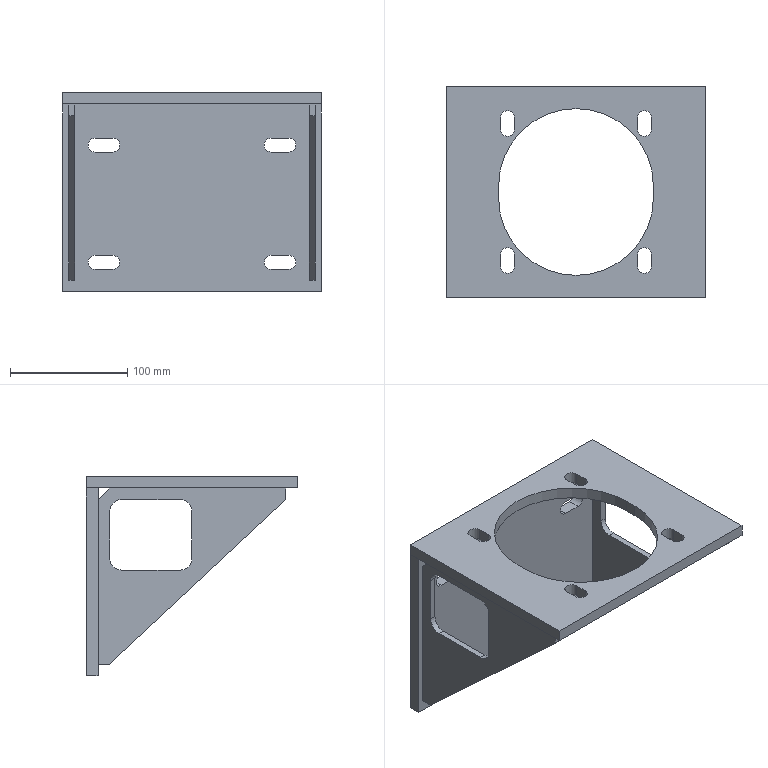Part | SolidWorks | features ICE 8, CirPattern 1, Extrusion 1, LPattern 1, MirrorSolid 1, WeldmentFeature 1 | 4 solids | 84 faces | box 220 x 180 x 170 mm | volume 670263 mm3 | plane 54 | cylinder 30 | commonest cylinder face diameters 12 x20 20 x8 132 x2